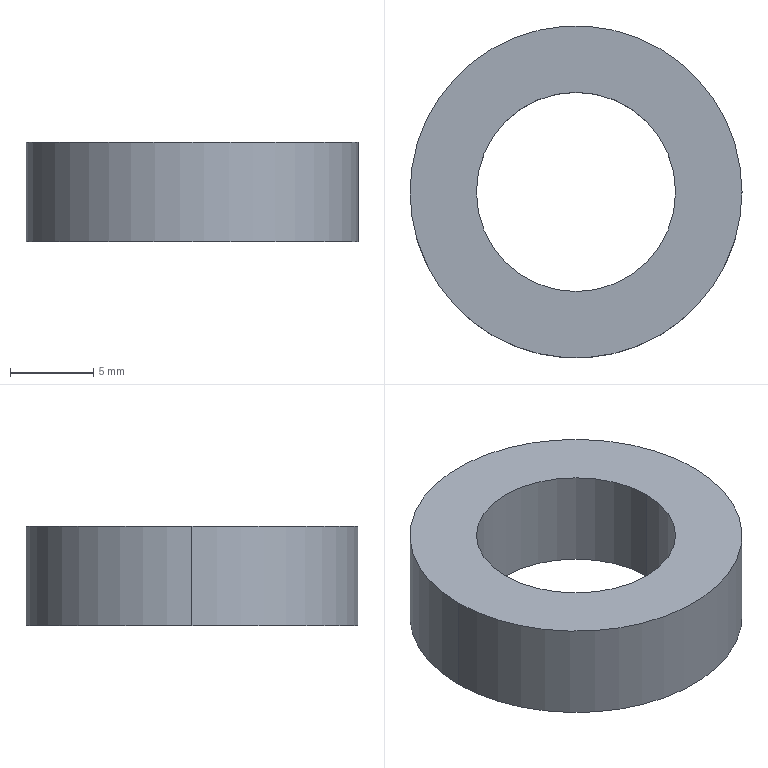Part | SolidWorks | features Extrusion 1 | 1 solid | 6 faces | box 20 x 20 x 6 mm | volume 1206 mm3 | cylinder 4 | plane 2 | commonest cylinder face diameters 12 x2 20 x2
STEP:
#1=CARTESIAN_POINT('',(-6.,0.,3.));
#2=VERTEX_POINT('',#1);
#3=CARTESIAN_POINT('',(6.,0.,3.));
#4=VERTEX_POINT('',#3);
#5=CARTESIAN_POINT('',(0.,0.,3.));
#6=DIRECTION('',(0.,0.,1.));
#7=DIRECTION('',(1.,0.,0.));
#8=AXIS2_PLACEMENT_3D('',#5,#6,#7);
#9=CIRCLE('',#8,6.);
#10=EDGE_CURVE('',#2,#4,#9,.T.);
#11=ORIENTED_EDGE('',*,*,#10,.T.);
#12=CARTESIAN_POINT('',(6.,0.,-3.));
#13=VERTEX_POINT('',#12);
#14=CARTESIAN_POINT('',(6.,0.,3.));
#15=DIRECTION('',(0.,0.,-1.));
#16=VECTOR('',#15,1000.);
#17=LINE('',#14,#16);
#18=EDGE_CURVE('',#4,#13,#17,.T.);
#19=ORIENTED_EDGE('',*,*,#18,.T.);
#20=CARTESIAN_POINT('',(-6.,0.,-3.));
#21=VERTEX_POINT('',#20);
#22=CARTESIAN_POINT('',(0.,0.,-3.));
#23=DIRECTION('',(0.,0.,1.));
#24=DIRECTION('',(1.,0.,0.));
#25=AXIS2_PLACEMENT_3D('',#22,#23,#24);
#26=CIRCLE('',#25,6.);
#27=EDGE_CURVE('',#21,#13,#26,.T.);
#28=ORIENTED_EDGE('',*,*,#27,.F.);
#29=CARTESIAN_POINT('',(-6.,0.,3.));
#30=DIRECTION('',(0.,0.,-1.));
#31=VECTOR('',#30,1000.);
#32=LINE('',#29,#31);
#33=EDGE_CURVE('',#2,#21,#32,.T.);
#34=ORIENTED_EDGE('',*,*,#33,.F.);
#35=EDGE_LOOP('',(#11,#19,#28,#34));
#36=FACE_OUTER_BOUND('',#35,.T.);
#37=CARTESIAN_POINT('',(0.,0.,3.));
#38=DIRECTION('',(0.,0.,-1.));
#39=DIRECTION('',(-1.,0.,0.));
#40=AXIS2_PLACEMENT_3D('',#37,#38,#39);
#41=CYLINDRICAL_SURFACE('',#40,6.);
#42=ADVANCED_FACE('',(#36),#41,.F.);
#43=CARTESIAN_POINT('',(10.,0.,3.));
#44=VERTEX_POINT('',#43);
#45=CARTESIAN_POINT('',(-10.,0.,3.));
#46=VERTEX_POINT('',#45);
#47=CARTESIAN_POINT('',(0.,0.,3.));
#48=DIRECTION('',(0.,0.,1.));
#49=DIRECTION('',(1.,0.,0.));
#50=AXIS2_PLACEMENT_3D('',#47,#48,#49);
#51=CIRCLE('',#50,10.);
#52=EDGE_CURVE('',#44,#46,#51,.T.);
#53=ORIENTED_EDGE('',*,*,#52,.F.);
#54=CARTESIAN_POINT('',(10.,0.,-3.));
#55=VERTEX_POINT('',#54);
#56=CARTESIAN_POINT('',(10.,0.,3.));
#57=DIRECTION('',(0.,0.,-1.));
#58=VECTOR('',#57,1000.);
#59=LINE('',#56,#58);
#60=EDGE_CURVE('',#44,#55,#59,.T.);
#61=ORIENTED_EDGE('',*,*,#60,.T.);
#62=CARTESIAN_POINT('',(-10.,0.,-3.));
#63=VERTEX_POINT('',#62);
#64=CARTESIAN_POINT('',(0.,0.,-3.));
#65=DIRECTION('',(0.,0.,1.));
#66=DIRECTION('',(1.,0.,0.));
#67=AXIS2_PLACEMENT_3D('',#64,#65,#66);
#68=CIRCLE('',#67,10.);
#69=EDGE_CURVE('',#55,#63,#68,.T.);
#70=ORIENTED_EDGE('',*,*,#69,.T.);
#71=CARTESIAN_POINT('',(-10.,0.,3.));
#72=DIRECTION('',(0.,0.,-1.));
#73=VECTOR('',#72,1000.);
#74=LINE('',#71,#73);
#75=EDGE_CURVE('',#46,#63,#74,.T.);
#76=ORIENTED_EDGE('',*,*,#75,.F.);
#77=EDGE_LOOP('',(#53,#61,#70,#76));
#78=FACE_OUTER_BOUND('',#77,.T.);
#79=CARTESIAN_POINT('',(0.,0.,3.));
#80=DIRECTION('',(0.,0.,-1.));
#81=DIRECTION('',(-1.,0.,0.));
#82=AXIS2_PLACEMENT_3D('',#79,#80,#81);
#83=CYLINDRICAL_SURFACE('',#82,10.);
#84=ADVANCED_FACE('',(#78),#83,.T.);
#85=CARTESIAN_POINT('',(0.,0.,3.));
#86=DIRECTION('',(0.,0.,1.));
#87=DIRECTION('',(1.,0.,0.));
#88=AXIS2_PLACEMENT_3D('',#85,#86,#87);
#89=CIRCLE('',#88,10.);
#90=EDGE_CURVE('',#46,#44,#89,.T.);
#91=ORIENTED_EDGE('',*,*,#90,.T.);
#92=ORIENTED_EDGE('',*,*,#52,.T.);
#93=EDGE_LOOP('',(#91,#92));
#94=FACE_OUTER_BOUND('',#93,.T.);
#95=ORIENTED_EDGE('',*,*,#10,.F.);
#96=CARTESIAN_POINT('',(0.,0.,3.));
#97=DIRECTION('',(0.,0.,1.));
#98=DIRECTION('',(1.,0.,0.));
#99=AXIS2_PLACEMENT_3D('',#96,#97,#98);
#100=CIRCLE('',#99,6.);
#101=EDGE_CURVE('',#4,#2,#100,.T.);
#102=ORIENTED_EDGE('',*,*,#101,.F.);
#103=EDGE_LOOP('',(#95,#102));
#104=FACE_BOUND('',#103,.T.);
#105=CARTESIAN_POINT('',(0.,0.,3.));
#106=DIRECTION('',(0.,0.,1.));
#107=DIRECTION('',(1.,0.,0.));
#108=AXIS2_PLACEMENT_3D('',#105,#106,#107);
#109=PLANE('',#108);
#110=ADVANCED_FACE('',(#94,#104),#109,.T.);
#111=CARTESIAN_POINT('',(0.,0.,-3.));
#112=DIRECTION('',(0.,0.,1.));
#113=DIRECTION('',(1.,0.,0.));
#114=AXIS2_PLACEMENT_3D('',#111,#112,#113);
#115=CIRCLE('',#114,10.);
#116=EDGE_CURVE('',#63,#55,#115,.T.);
#117=ORIENTED_EDGE('',*,*,#116,.F.);
#118=ORIENTED_EDGE('',*,*,#69,.F.);
#119=EDGE_LOOP('',(#117,#118));
#120=FACE_OUTER_BOUND('',#119,.T.);
#121=ORIENTED_EDGE('',*,*,#27,.T.);
#122=CARTESIAN_POINT('',(0.,0.,-3.));
#123=DIRECTION('',(0.,0.,1.));
#124=DIRECTION('',(1.,0.,0.));
#125=AXIS2_PLACEMENT_3D('',#122,#123,#124);
#126=CIRCLE('',#125,6.);
#127=EDGE_CURVE('',#13,#21,#126,.T.);
#128=ORIENTED_EDGE('',*,*,#127,.T.);
#129=EDGE_LOOP('',(#121,#128));
#130=FACE_BOUND('',#129,.T.);
#131=CARTESIAN_POINT('',(0.,0.,-3.));
#132=DIRECTION('',(0.,0.,1.));
#133=DIRECTION('',(1.,0.,0.));
#134=AXIS2_PLACEMENT_3D('',#131,#132,#133);
#135=PLANE('',#134);
#136=ADVANCED_FACE('',(#120,#130),#135,.F.);
#137=ORIENTED_EDGE('',*,*,#60,.F.);
#138=ORIENTED_EDGE('',*,*,#90,.F.);
#139=ORIENTED_EDGE('',*,*,#75,.T.);
#140=ORIENTED_EDGE('',*,*,#116,.T.);
#141=EDGE_LOOP('',(#137,#138,#139,#140));
#142=FACE_OUTER_BOUND('',#141,.T.);
#143=CARTESIAN_POINT('',(0.,0.,3.));
#144=DIRECTION('',(0.,0.,-1.));
#145=DIRECTION('',(-1.,0.,0.));
#146=AXIS2_PLACEMENT_3D('',#143,#144,#145);
#147=CYLINDRICAL_SURFACE('',#146,10.);
#148=ADVANCED_FACE('',(#142),#147,.T.);
#149=ORIENTED_EDGE('',*,*,#18,.F.);
#150=ORIENTED_EDGE('',*,*,#101,.T.);
#151=ORIENTED_EDGE('',*,*,#33,.T.);
#152=ORIENTED_EDGE('',*,*,#127,.F.);
#153=EDGE_LOOP('',(#149,#150,#151,#152));
#154=FACE_OUTER_BOUND('',#153,.T.);
#155=CARTESIAN_POINT('',(0.,0.,3.));
#156=DIRECTION('',(0.,0.,-1.));
#157=DIRECTION('',(-1.,0.,0.));
#158=AXIS2_PLACEMENT_3D('',#155,#156,#157);
#159=CYLINDRICAL_SURFACE('',#158,6.);
#160=ADVANCED_FACE('',(#154),#159,.F.);
#161=CLOSED_SHELL('',(#42,#84,#110,#136,#148,#160));
#162=MANIFOLD_SOLID_BREP('',#161);
#163=CARTESIAN_POINT('',(0.,0.,0.));
#164=DIRECTION('',(0.,0.,1.));
#165=DIRECTION('',(1.,0.,0.));
#166=AXIS2_PLACEMENT_3D('',#163,#164,#165);
#167=(LENGTH_UNIT()NAMED_UNIT(*)SI_UNIT(.MILLI.,.METRE.));
#168=UNCERTAINTY_MEASURE_WITH_UNIT(LENGTH_MEASURE(0.00001),#167,'','');
#169=(NAMED_UNIT(*)PLANE_ANGLE_UNIT()SI_UNIT($,.RADIAN.));
#170=(NAMED_UNIT(*)SI_UNIT($,.STERADIAN.)SOLID_ANGLE_UNIT());
#171=(GEOMETRIC_REPRESENTATION_CONTEXT(3)GLOBAL_UNCERTAINTY_ASSIGNED_CONTEXT((#168))GLOBAL_UNIT_ASSIGNED_CONTEXT((#167,#169,#170))REPRESENTATION_CONTEXT('',''));
#172=ADVANCED_BREP_SHAPE_REPRESENTATION('',(#162,#166),#171);